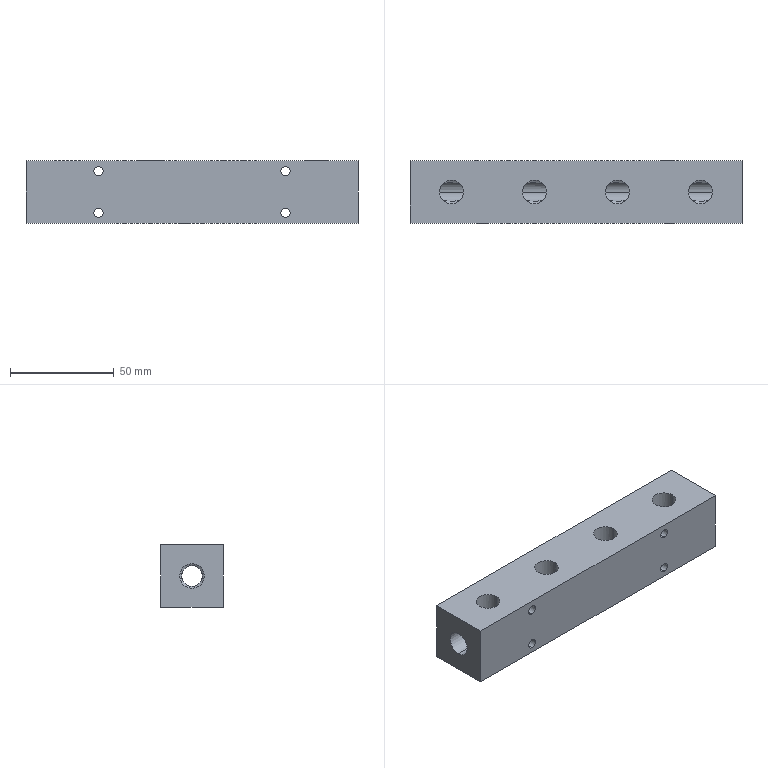Part | SolidWorks | features BaseBody 1 | 1 solid | 56 faces | box 160 x 30 x 30 mm | volume 122466 mm3 | cylinder 32 | cone 14 | plane 10 | commonest cylinder face diameters 4.5 x8 8 x8 11.445 x8 11.8 x6 10 x2